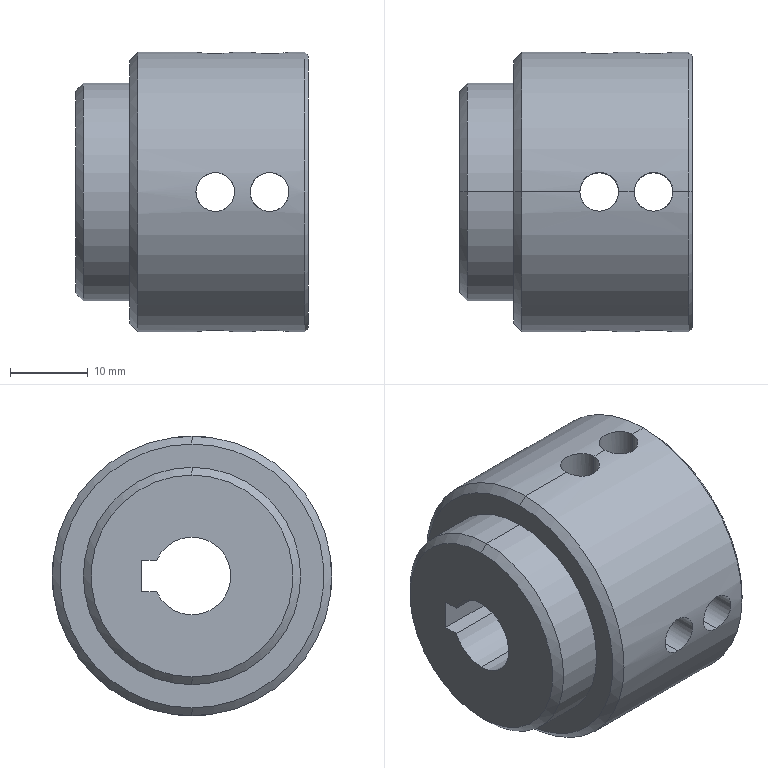Part | SolidWorks | features ICE 3, Chamfer 2, Revolution 1 | 1 solid | 40 faces | box 30 x 36 x 36 mm | volume 17490 mm3 | cylinder 25 | cone 8 | plane 7 | commonest cylinder face diameters 5 x16 10 x3 24 x2 28 x2 36 x2